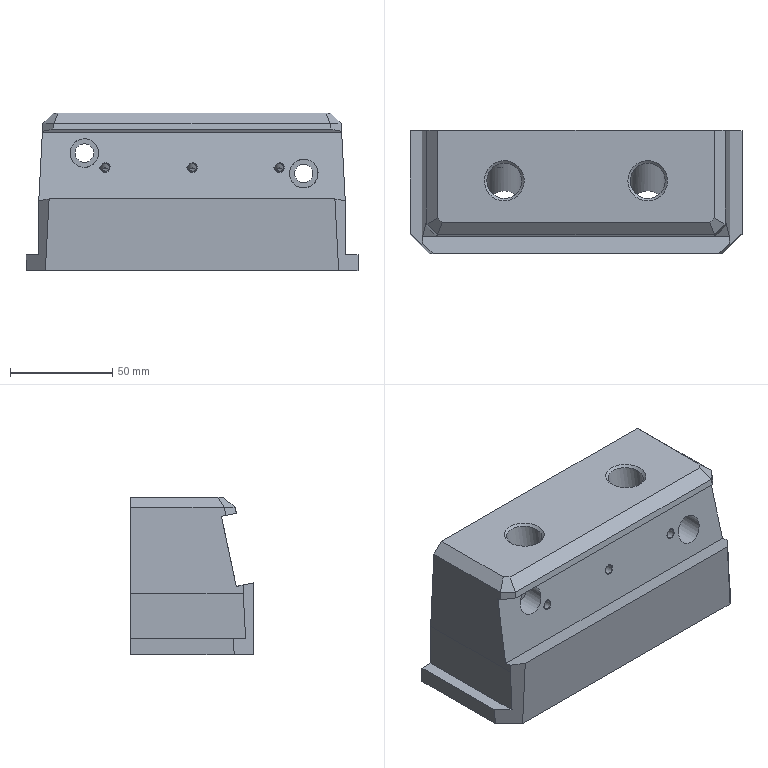Part | STEP file | P011002S004-000 | 1 solid | 162 faces | box 162 x 60 x 77 mm | volume 547857 mm3 | plane 105 | cylinder 25 | cone 15 | other 15 | spline 2 | commonest cylinder face diameters 6 x8 4.167 x3 4.983 x3 5 x3 9 x2 13 x2